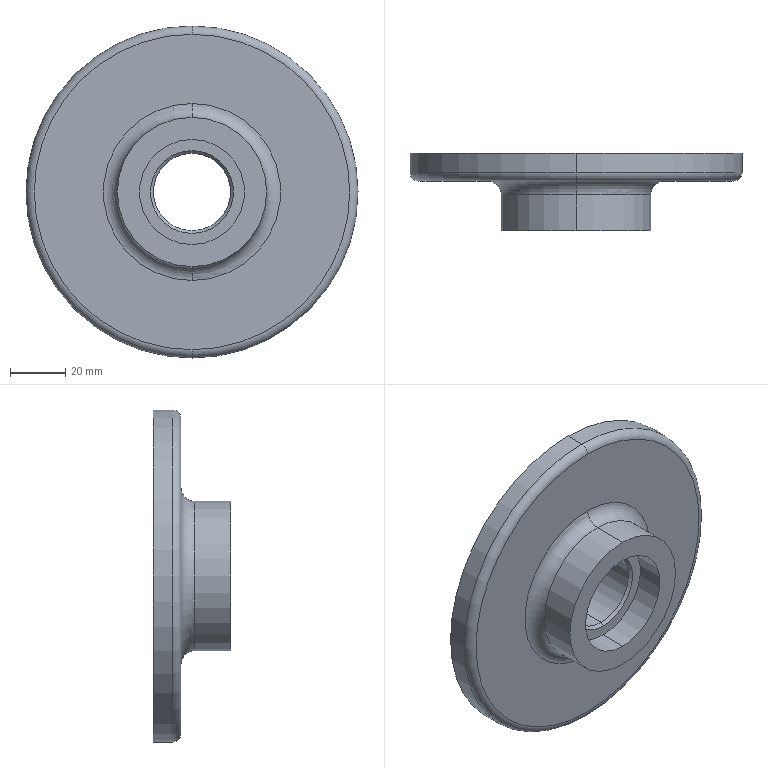Part | NX | features BREP 1 | 1 solid | 44 faces | box 120 x 27.99 x 120 mm | volume 131699 mm3 | cylinder 20 | cone 16 | torus 4 | plane 4 | commonest cylinder face diameters 3.3 x12 28 x2 38 x2 54 x2 120 x2
STEP:
#1=CARTESIAN_POINT('',(-56.,4.13,-1.65));
#2=VERTEX_POINT('',#1);
#3=CARTESIAN_POINT('',(-56.,4.13,1.65));
#4=VERTEX_POINT('',#3);
#5=CARTESIAN_POINT('',(-56.,4.13,0.));
#6=DIRECTION('',(0.,1.,0.));
#7=DIRECTION('',(0.,0.,1.));
#8=AXIS2_PLACEMENT_3D('',#5,#6,#7);
#9=CIRCLE('',#8,1.65);
#10=EDGE_CURVE('',#2,#4,#9,.T.);
#11=ORIENTED_EDGE('',*,*,#10,.F.);
#12=CARTESIAN_POINT('',(-56.,10.,-1.65));
#13=VERTEX_POINT('',#12);
#14=CARTESIAN_POINT('',(-56.,10.,-1.65));
#15=DIRECTION('',(0.,1.,0.));
#16=VECTOR('',#15,1000.);
#17=LINE('',#14,#16);
#18=EDGE_CURVE('',#2,#13,#17,.T.);
#19=ORIENTED_EDGE('',*,*,#18,.T.);
#20=CARTESIAN_POINT('',(-56.,10.,1.65));
#21=VERTEX_POINT('',#20);
#22=CARTESIAN_POINT('',(-56.,10.,0.));
#23=DIRECTION('',(0.,1.,0.));
#24=DIRECTION('',(0.,0.,1.));
#25=AXIS2_PLACEMENT_3D('',#22,#23,#24);
#26=CIRCLE('',#25,1.65);
#27=EDGE_CURVE('',#13,#21,#26,.T.);
#28=ORIENTED_EDGE('',*,*,#27,.T.);
#29=CARTESIAN_POINT('',(-56.,10.,1.65));
#30=DIRECTION('',(0.,1.,0.));
#31=VECTOR('',#30,1000.);
#32=LINE('',#29,#31);
#33=EDGE_CURVE('',#4,#21,#32,.T.);
#34=ORIENTED_EDGE('',*,*,#33,.F.);
#35=EDGE_LOOP('',(#11,#19,#28,#34));
#36=FACE_BOUND('',#35,.T.);
#37=CARTESIAN_POINT('',(-56.,10.,0.));
#38=DIRECTION('',(0.,1.,0.));
#39=DIRECTION('',(0.,0.,-1.));
#40=AXIS2_PLACEMENT_3D('',#37,#38,#39);
#41=CYLINDRICAL_SURFACE('',#40,1.65);
#42=ADVANCED_FACE('',(#36),#41,.F.);
#43=CARTESIAN_POINT('',(-56.,3.139,0.));
#44=VERTEX_POINT('',#43);
#45=CARTESIAN_POINT('',(-56.,4.13,1.65));
#46=DIRECTION('',(0.,0.515,0.8572));
#47=VECTOR('',#46,1000.);
#48=LINE('',#45,#47);
#49=EDGE_CURVE('',#44,#4,#48,.T.);
#50=ORIENTED_EDGE('',*,*,#49,.F.);
#51=CARTESIAN_POINT('',(-56.,4.13,-1.65));
#52=DIRECTION('',(0.,0.515,-0.8572));
#53=VECTOR('',#52,1000.);
#54=LINE('',#51,#53);
#55=EDGE_CURVE('',#44,#2,#54,.T.);
#56=ORIENTED_EDGE('',*,*,#55,.T.);
#57=ORIENTED_EDGE('',*,*,#10,.T.);
#58=EDGE_LOOP('',(#50,#56,#57));
#59=FACE_BOUND('',#58,.T.);
#60=CARTESIAN_POINT('',(-56.,4.13,0.));
#61=DIRECTION('',(0.,1.,0.));
#62=DIRECTION('',(0.,0.,-1.));
#63=AXIS2_PLACEMENT_3D('',#60,#61,#62);
#64=CONICAL_SURFACE('',#63,1.65,1.03);
#65=ADVANCED_FACE('',(#59),#64,.F.);
#66=CARTESIAN_POINT('',(-28.,4.13,-50.147));
#67=VERTEX_POINT('',#66);
#68=CARTESIAN_POINT('',(-28.,4.13,-46.847));
#69=VERTEX_POINT('',#68);
#70=CARTESIAN_POINT('',(-28.,4.13,-48.497));
#71=DIRECTION('',(0.,1.,0.));
#72=DIRECTION('',(0.,0.,1.));
#73=AXIS2_PLACEMENT_3D('',#70,#71,#72);
#74=CIRCLE('',#73,1.65);
#75=EDGE_CURVE('',#67,#69,#74,.T.);
#76=ORIENTED_EDGE('',*,*,#75,.F.);
#77=CARTESIAN_POINT('',(-28.,10.,-50.147));
#78=VERTEX_POINT('',#77);
#79=CARTESIAN_POINT('',(-28.,10.,-50.147));
#80=DIRECTION('',(0.,1.,0.));
#81=VECTOR('',#80,1000.);
#82=LINE('',#79,#81);
#83=EDGE_CURVE('',#67,#78,#82,.T.);
#84=ORIENTED_EDGE('',*,*,#83,.T.);
#85=CARTESIAN_POINT('',(-28.,10.,-46.847));
#86=VERTEX_POINT('',#85);
#87=CARTESIAN_POINT('',(-28.,10.,-48.497));
#88=DIRECTION('',(0.,1.,0.));
#89=DIRECTION('',(0.,0.,1.));
#90=AXIS2_PLACEMENT_3D('',#87,#88,#89);
#91=CIRCLE('',#90,1.65);
#92=EDGE_CURVE('',#78,#86,#91,.T.);
#93=ORIENTED_EDGE('',*,*,#92,.T.);
#94=CARTESIAN_POINT('',(-28.,10.,-46.847));
#95=DIRECTION('',(0.,1.,0.));
#96=VECTOR('',#95,1000.);
#97=LINE('',#94,#96);
#98=EDGE_CURVE('',#69,#86,#97,.T.);
#99=ORIENTED_EDGE('',*,*,#98,.F.);
#100=EDGE_LOOP('',(#76,#84,#93,#99));
#101=FACE_BOUND('',#100,.T.);
#102=CARTESIAN_POINT('',(-28.,10.,-48.497));
#103=DIRECTION('',(0.,1.,0.));
#104=DIRECTION('',(0.,0.,-1.));
#105=AXIS2_PLACEMENT_3D('',#102,#103,#104);
#106=CYLINDRICAL_SURFACE('',#105,1.65);
#107=ADVANCED_FACE('',(#101),#106,.F.);
#108=CARTESIAN_POINT('',(-28.,3.139,-48.497));
#109=VERTEX_POINT('',#108);
#110=CARTESIAN_POINT('',(-28.,4.13,-46.847));
#111=DIRECTION('',(0.,0.515,0.8572));
#112=VECTOR('',#111,1000.);
#113=LINE('',#110,#112);
#114=EDGE_CURVE('',#109,#69,#113,.T.);
#115=ORIENTED_EDGE('',*,*,#114,.F.);
#116=CARTESIAN_POINT('',(-28.,4.13,-50.147));
#117=DIRECTION('',(0.,0.515,-0.8572));
#118=VECTOR('',#117,1000.);
#119=LINE('',#116,#118);
#120=EDGE_CURVE('',#109,#67,#119,.T.);
#121=ORIENTED_EDGE('',*,*,#120,.T.);
#122=ORIENTED_EDGE('',*,*,#75,.T.);
#123=EDGE_LOOP('',(#115,#121,#122));
#124=FACE_BOUND('',#123,.T.);
#125=CARTESIAN_POINT('',(-28.,4.13,-48.497));
#126=DIRECTION('',(0.,1.,0.));
#127=DIRECTION('',(0.,0.,-1.));
#128=AXIS2_PLACEMENT_3D('',#125,#126,#127);
#129=CONICAL_SURFACE('',#128,1.65,1.03);
#130=ADVANCED_FACE('',(#124),#129,.F.);
#131=CARTESIAN_POINT('',(28.,4.13,-50.147));
#132=VERTEX_POINT('',#131);
#133=CARTESIAN_POINT('',(28.,4.13,-46.847));
#134=VERTEX_POINT('',#133);
#135=CARTESIAN_POINT('',(28.,4.13,-48.497));
#136=DIRECTION('',(0.,1.,0.));
#137=DIRECTION('',(0.,0.,1.));
#138=AXIS2_PLACEMENT_3D('',#135,#136,#137);
#139=CIRCLE('',#138,1.65);
#140=EDGE_CURVE('',#132,#134,#139,.T.);
#141=ORIENTED_EDGE('',*,*,#140,.F.);
#142=CARTESIAN_POINT('',(28.,10.,-50.147));
#143=VERTEX_POINT('',#142);
#144=CARTESIAN_POINT('',(28.,10.,-50.147));
#145=DIRECTION('',(0.,1.,0.));
#146=VECTOR('',#145,1000.);
#147=LINE('',#144,#146);
#148=EDGE_CURVE('',#132,#143,#147,.T.);
#149=ORIENTED_EDGE('',*,*,#148,.T.);
#150=CARTESIAN_POINT('',(28.,10.,-46.847));
#151=VERTEX_POINT('',#150);
#152=CARTESIAN_POINT('',(28.,10.,-48.497));
#153=DIRECTION('',(0.,1.,0.));
#154=DIRECTION('',(0.,0.,1.));
#155=AXIS2_PLACEMENT_3D('',#152,#153,#154);
#156=CIRCLE('',#155,1.65);
#157=EDGE_CURVE('',#143,#151,#156,.T.);
#158=ORIENTED_EDGE('',*,*,#157,.T.);
#159=CARTESIAN_POINT('',(28.,10.,-46.847));
#160=DIRECTION('',(0.,1.,0.));
#161=VECTOR('',#160,1000.);
#162=LINE('',#159,#161);
#163=EDGE_CURVE('',#134,#151,#162,.T.);
#164=ORIENTED_EDGE('',*,*,#163,.F.);
#165=EDGE_LOOP('',(#141,#149,#158,#164));
#166=FACE_BOUND('',#165,.T.);
#167=CARTESIAN_POINT('',(28.,10.,-48.497));
#168=DIRECTION('',(0.,1.,0.));
#169=DIRECTION('',(0.,0.,-1.));
#170=AXIS2_PLACEMENT_3D('',#167,#168,#169);
#171=CYLINDRICAL_SURFACE('',#170,1.65);
#172=ADVANCED_FACE('',(#166),#171,.F.);
#173=CARTESIAN_POINT('',(28.,3.139,-48.497));
#174=VERTEX_POINT('',#173);
#175=CARTESIAN_POINT('',(28.,4.13,-46.847));
#176=DIRECTION('',(0.,0.515,0.8572));
#177=VECTOR('',#176,1000.);
#178=LINE('',#175,#177);
#179=EDGE_CURVE('',#174,#134,#178,.T.);
#180=ORIENTED_EDGE('',*,*,#179,.F.);
#181=CARTESIAN_POINT('',(28.,4.13,-50.147));
#182=DIRECTION('',(0.,0.515,-0.8572));
#183=VECTOR('',#182,1000.);
#184=LINE('',#181,#183);
#185=EDGE_CURVE('',#174,#132,#184,.T.);
#186=ORIENTED_EDGE('',*,*,#185,.T.);
#187=ORIENTED_EDGE('',*,*,#140,.T.);
#188=EDGE_LOOP('',(#180,#186,#187));
#189=FACE_BOUND('',#188,.T.);
#190=CARTESIAN_POINT('',(28.,4.13,-48.497));
#191=DIRECTION('',(0.,1.,0.));
#192=DIRECTION('',(0.,0.,-1.));
#193=AXIS2_PLACEMENT_3D('',#190,#191,#192);
#194=CONICAL_SURFACE('',#193,1.65,1.03);
#195=ADVANCED_FACE('',(#189),#194,.F.);
#196=CARTESIAN_POINT('',(56.,4.13,-1.65));
#197=VERTEX_POINT('',#196);
#198=CARTESIAN_POINT('',(56.,4.13,1.65));
#199=VERTEX_POINT('',#198);
#200=CARTESIAN_POINT('',(56.,4.13,0.));
#201=DIRECTION('',(0.,1.,0.));
#202=DIRECTION('',(0.,0.,1.));
#203=AXIS2_PLACEMENT_3D('',#200,#201,#202);
#204=CIRCLE('',#203,1.65);
#205=EDGE_CURVE('',#197,#199,#204,.T.);
#206=ORIENTED_EDGE('',*,*,#205,.F.);
#207=CARTESIAN_POINT('',(56.,10.,-1.65));
#208=VERTEX_POINT('',#207);
#209=CARTESIAN_POINT('',(56.,10.,-1.65));
#210=DIRECTION('',(0.,1.,0.));
#211=VECTOR('',#210,1000.);
#212=LINE('',#209,#211);
#213=EDGE_CURVE('',#197,#208,#212,.T.);
#214=ORIENTED_EDGE('',*,*,#213,.T.);
#215=CARTESIAN_POINT('',(56.,10.,1.65));
#216=VERTEX_POINT('',#215);
#217=CARTESIAN_POINT('',(56.,10.,0.));
#218=DIRECTION('',(0.,1.,0.));
#219=DIRECTION('',(0.,0.,1.));
#220=AXIS2_PLACEMENT_3D('',#217,#218,#219);
#221=CIRCLE('',#220,1.65);
#222=EDGE_CURVE('',#208,#216,#221,.T.);
#223=ORIENTED_EDGE('',*,*,#222,.T.);
#224=CARTESIAN_POINT('',(56.,10.,1.65));
#225=DIRECTION('',(0.,1.,0.));
#226=VECTOR('',#225,1000.);
#227=LINE('',#224,#226);
#228=EDGE_CURVE('',#199,#216,#227,.T.);
#229=ORIENTED_EDGE('',*,*,#228,.F.);
#230=EDGE_LOOP('',(#206,#214,#223,#229));
#231=FACE_BOUND('',#230,.T.);
#232=CARTESIAN_POINT('',(56.,10.,0.));
#233=DIRECTION('',(0.,1.,0.));
#234=DIRECTION('',(0.,0.,-1.));
#235=AXIS2_PLACEMENT_3D('',#232,#233,#234);
#236=CYLINDRICAL_SURFACE('',#235,1.65);
#237=ADVANCED_FACE('',(#231),#236,.F.);
#238=CARTESIAN_POINT('',(56.,3.139,0.));
#239=VERTEX_POINT('',#238);
#240=CARTESIAN_POINT('',(56.,4.13,1.65));
#241=DIRECTION('',(0.,0.515,0.8572));
#242=VECTOR('',#241,1000.);
#243=LINE('',#240,#242);
#244=EDGE_CURVE('',#239,#199,#243,.T.);
#245=ORIENTED_EDGE('',*,*,#244,.F.);
#246=CARTESIAN_POINT('',(56.,4.13,-1.65));
#247=DIRECTION('',(0.,0.515,-0.8572));
#248=VECTOR('',#247,1000.);
#249=LINE('',#246,#248);
#250=EDGE_CURVE('',#239,#197,#249,.T.);
#251=ORIENTED_EDGE('',*,*,#250,.T.);
#252=ORIENTED_EDGE('',*,*,#205,.T.);
#253=EDGE_LOOP('',(#245,#251,#252));
#254=FACE_BOUND('',#253,.T.);
#255=CARTESIAN_POINT('',(56.,4.13,0.));
#256=DIRECTION('',(0.,1.,0.));
#257=DIRECTION('',(0.,0.,-1.));
#258=AXIS2_PLACEMENT_3D('',#255,#256,#257);
#259=CONICAL_SURFACE('',#258,1.65,1.03);
#260=ADVANCED_FACE('',(#254),#259,.F.);
#261=CARTESIAN_POINT('',(28.,4.13,46.847));
#262=VERTEX_POINT('',#261);
#263=CARTESIAN_POINT('',(28.,4.13,50.147));
#264=VERTEX_POINT('',#263);
#265=CARTESIAN_POINT('',(28.,4.13,48.497));
#266=DIRECTION('',(0.,1.,0.));
#267=DIRECTION('',(0.,0.,1.));
#268=AXIS2_PLACEMENT_3D('',#265,#266,#267);
#269=CIRCLE('',#268,1.65);
#270=EDGE_CURVE('',#262,#264,#269,.T.);
#271=ORIENTED_EDGE('',*,*,#270,.F.);
#272=CARTESIAN_POINT('',(28.,10.,46.847));
#273=VERTEX_POINT('',#272);
#274=CARTESIAN_POINT('',(28.,10.,46.847));
#275=DIRECTION('',(0.,1.,0.));
#276=VECTOR('',#275,1000.);
#277=LINE('',#274,#276);
#278=EDGE_CURVE('',#262,#273,#277,.T.);
#279=ORIENTED_EDGE('',*,*,#278,.T.);
#280=CARTESIAN_POINT('',(28.,10.,50.147));
#281=VERTEX_POINT('',#280);
#282=CARTESIAN_POINT('',(28.,10.,48.497));
#283=DIRECTION('',(0.,1.,0.));
#284=DIRECTION('',(0.,0.,1.));
#285=AXIS2_PLACEMENT_3D('',#282,#283,#284);
#286=CIRCLE('',#285,1.65);
#287=EDGE_CURVE('',#273,#281,#286,.T.);
#288=ORIENTED_EDGE('',*,*,#287,.T.);
#289=CARTESIAN_POINT('',(28.,10.,50.147));
#290=DIRECTION('',(0.,1.,0.));
#291=VECTOR('',#290,1000.);
#292=LINE('',#289,#291);
#293=EDGE_CURVE('',#264,#281,#292,.T.);
#294=ORIENTED_EDGE('',*,*,#293,.F.);
#295=EDGE_LOOP('',(#271,#279,#288,#294));
#296=FACE_BOUND('',#295,.T.);
#297=CARTESIAN_POINT('',(28.,10.,48.497));
#298=DIRECTION('',(0.,1.,0.));
#299=DIRECTION('',(0.,0.,-1.));
#300=AXIS2_PLACEMENT_3D('',#297,#298,#299);
#301=CYLINDRICAL_SURFACE('',#300,1.65);
#302=ADVANCED_FACE('',(#296),#301,.F.);
#303=CARTESIAN_POINT('',(28.,3.139,48.497));
#304=VERTEX_POINT('',#303);
#305=CARTESIAN_POINT('',(28.,4.13,50.147));
#306=DIRECTION('',(0.,0.515,0.8572));
#307=VECTOR('',#306,1000.);
#308=LINE('',#305,#307);
#309=EDGE_CURVE('',#304,#264,#308,.T.);
#310=ORIENTED_EDGE('',*,*,#309,.F.);
#311=CARTESIAN_POINT('',(28.,4.13,46.847));
#312=DIRECTION('',(0.,0.515,-0.8572));
#313=VECTOR('',#312,1000.);
#314=LINE('',#311,#313);
#315=EDGE_CURVE('',#304,#262,#314,.T.);
#316=ORIENTED_EDGE('',*,*,#315,.T.);
#317=ORIENTED_EDGE('',*,*,#270,.T.);
#318=EDGE_LOOP('',(#310,#316,#317));
#319=FACE_BOUND('',#318,.T.);
#320=CARTESIAN_POINT('',(28.,4.13,48.497));
#321=DIRECTION('',(0.,1.,0.));
#322=DIRECTION('',(0.,0.,-1.));
#323=AXIS2_PLACEMENT_3D('',#320,#321,#322);
#324=CONICAL_SURFACE('',#323,1.65,1.03);
#325=ADVANCED_FACE('',(#319),#324,.F.);
#326=CARTESIAN_POINT('',(-28.,4.13,46.847));
#327=VERTEX_POINT('',#326);
#328=CARTESIAN_POINT('',(-28.,4.13,50.147));
#329=VERTEX_POINT('',#328);
#330=CARTESIAN_POINT('',(-28.,4.13,48.497));
#331=DIRECTION('',(0.,1.,0.));
#332=DIRECTION('',(0.,0.,1.));
#333=AXIS2_PLACEMENT_3D('',#330,#331,#332);
#334=CIRCLE('',#333,1.65);
#335=EDGE_CURVE('',#327,#329,#334,.T.);
#336=ORIENTED_EDGE('',*,*,#335,.F.);
#337=CARTESIAN_POINT('',(-28.,10.,46.847));
#338=VERTEX_POINT('',#337);
#339=CARTESIAN_POINT('',(-28.,10.,46.847));
#340=DIRECTION('',(0.,1.,0.));
#341=VECTOR('',#340,1000.);
#342=LINE('',#339,#341);
#343=EDGE_CURVE('',#327,#338,#342,.T.);
#344=ORIENTED_EDGE('',*,*,#343,.T.);
#345=CARTESIAN_POINT('',(-28.,10.,50.147));
#346=VERTEX_POINT('',#345);
#347=CARTESIAN_POINT('',(-28.,10.,48.497));
#348=DIRECTION('',(0.,1.,0.));
#349=DIRECTION('',(0.,0.,1.));
#350=AXIS2_PLACEMENT_3D('',#347,#348,#349);
#351=CIRCLE('',#350,1.65);
#352=EDGE_CURVE('',#338,#346,#351,.T.);
#353=ORIENTED_EDGE('',*,*,#352,.T.);
#354=CARTESIAN_POINT('',(-28.,10.,50.147));
#355=DIRECTION('',(0.,1.,0.));
#356=VECTOR('',#355,1000.);
#357=LINE('',#354,#356);
#358=EDGE_CURVE('',#329,#346,#357,.T.);
#359=ORIENTED_EDGE('',*,*,#358,.F.);
#360=EDGE_LOOP('',(#336,#344,#353,#359));
#361=FACE_BOUND('',#360,.T.);
#362=CARTESIAN_POINT('',(-28.,10.,48.497));
#363=DIRECTION('',(0.,1.,0.));
#364=DIRECTION('',(0.,0.,-1.));
#365=AXIS2_PLACEMENT_3D('',#362,#363,#364);
#366=CYLINDRICAL_SURFACE('',#365,1.65);
#367=ADVANCED_FACE('',(#361),#366,.F.);
#368=CARTESIAN_POINT('',(-28.,3.139,48.497));
#369=VERTEX_POINT('',#368);
#370=CARTESIAN_POINT('',(-28.,4.13,50.147));
#371=DIRECTION('',(0.,0.515,0.8572));
#372=VECTOR('',#371,1000.);
#373=LINE('',#370,#372);
#374=EDGE_CURVE('',#369,#329,#373,.T.);
#375=ORIENTED_EDGE('',*,*,#374,.F.);
#376=CARTESIAN_POINT('',(-28.,4.13,46.847));
#377=DIRECTION('',(0.,0.515,-0.8572));
#378=VECTOR('',#377,1000.);
#379=LINE('',#376,#378);
#380=EDGE_CURVE('',#369,#327,#379,.T.);
#381=ORIENTED_EDGE('',*,*,#380,.T.);
#382=ORIENTED_EDGE('',*,*,#335,.T.);
#383=EDGE_LOOP('',(#375,#381,#382));
#384=FACE_BOUND('',#383,.T.);
#385=CARTESIAN_POINT('',(-28.,4.13,48.497));
#386=DIRECTION('',(0.,1.,0.));
#387=DIRECTION('',(0.,0.,-1.));
#388=AXIS2_PLACEMENT_3D('',#385,#386,#387);
#389=CONICAL_SURFACE('',#388,1.65,1.03);
#390=ADVANCED_FACE('',(#384),#389,.F.);
#391=CARTESIAN_POINT('',(0.,0.,57.));
#392=VERTEX_POINT('',#391);
#393=CARTESIAN_POINT('',(0.,0.,-57.));
#394=VERTEX_POINT('',#393);
#395=CARTESIAN_POINT('',(0.,0.,0.));
#396=DIRECTION('',(0.,1.,0.));
#397=DIRECTION('',(0.,0.,1.));
#398=AXIS2_PLACEMENT_3D('',#395,#396,#397);
#399=CIRCLE('',#398,57.);
#400=EDGE_CURVE('',#392,#394,#399,.T.);
#401=ORIENTED_EDGE('',*,*,#400,.T.);
#402=CARTESIAN_POINT('',(0.,3.,-60.));
#403=VERTEX_POINT('',#402);
#404=CARTESIAN_POINT('',(0.,3.,-57.));
#405=DIRECTION('',(1.,0.,0.));
#406=DIRECTION('',(0.,0.,-1.));
#407=AXIS2_PLACEMENT_3D('',#404,#405,#406);
#408=CIRCLE('',#407,3.);
#409=EDGE_CURVE('',#394,#403,#408,.T.);
#410=ORIENTED_EDGE('',*,*,#409,.T.);
#411=CARTESIAN_POINT('',(0.,3.,60.));
#412=VERTEX_POINT('',#411);
#413=CARTESIAN_POINT('',(0.,3.,0.));
#414=DIRECTION('',(0.,1.,0.));
#415=DIRECTION('',(0.,0.,1.));
#416=AXIS2_PLACEMENT_3D('',#413,#414,#415);
#417=CIRCLE('',#416,60.);
#418=EDGE_CURVE('',#412,#403,#417,.T.);
#419=ORIENTED_EDGE('',*,*,#418,.F.);
#420=CARTESIAN_POINT('',(0.,3.,57.));
#421=DIRECTION('',(-1.,0.,0.));
#422=DIRECTION('',(0.,0.,1.));
#423=AXIS2_PLACEMENT_3D('',#420,#421,#422);
#424=CIRCLE('',#423,3.);
#425=EDGE_CURVE('',#392,#412,#424,.T.);
#426=ORIENTED_EDGE('',*,*,#425,.F.);
#427=EDGE_LOOP('',(#401,#410,#419,#426));
#428=FACE_BOUND('',#427,.T.);
#429=CARTESIAN_POINT('',(0.,3.,0.));
#430=DIRECTION('',(0.,1.,0.));
#431=DIRECTION('',(0.,0.,-1.));
#432=AXIS2_PLACEMENT_3D('',#429,#430,#431);
#433=TOROIDAL_SURFACE('',#432,57.,3.);
#434=ADVANCED_FACE('',(#428),#433,.T.);
#435=CARTESIAN_POINT('',(0.,0.,-32.));
#436=VERTEX_POINT('',#435);
#437=CARTESIAN_POINT('',(0.,0.,32.));
#438=VERTEX_POINT('',#437);
#439=CARTESIAN_POINT('',(0.,0.,0.));
#440=DIRECTION('',(0.,1.,0.));
#441=DIRECTION('',(0.,0.,1.));
#442=AXIS2_PLACEMENT_3D('',#439,#440,#441);
#443=CIRCLE('',#442,32.);
#444=EDGE_CURVE('',#436,#438,#443,.T.);
#445=ORIENTED_EDGE('',*,*,#444,.F.);
#446=CARTESIAN_POINT('',(0.,-5.,-27.));
#447=VERTEX_POINT('',#446);
#448=CARTESIAN_POINT('',(0.,-5.,-32.));
#449=DIRECTION('',(1.,0.,0.));
#450=DIRECTION('',(0.,0.,-1.));
#451=AXIS2_PLACEMENT_3D('',#448,#449,#450);
#452=CIRCLE('',#451,5.);
#453=EDGE_CURVE('',#436,#447,#452,.T.);
#454=ORIENTED_EDGE('',*,*,#453,.T.);
#455=CARTESIAN_POINT('',(0.,-5.,27.));
#456=VERTEX_POINT('',#455);
#457=CARTESIAN_POINT('',(0.,-5.,0.));
#458=DIRECTION('',(0.,1.,0.));
#459=DIRECTION('',(0.,0.,1.));
#460=AXIS2_PLACEMENT_3D('',#457,#458,#459);
#461=CIRCLE('',#460,27.);
#462=EDGE_CURVE('',#447,#456,#461,.T.);
#463=ORIENTED_EDGE('',*,*,#462,.T.);
#464=CARTESIAN_POINT('',(0.,-5.,32.));
#465=DIRECTION('',(-1.,0.,0.));
#466=DIRECTION('',(0.,0.,1.));
#467=AXIS2_PLACEMENT_3D('',#464,#465,#466);
#468=CIRCLE('',#467,5.);
#469=EDGE_CURVE('',#438,#456,#468,.T.);
#470=ORIENTED_EDGE('',*,*,#469,.F.);
#471=EDGE_LOOP('',(#445,#454,#463,#470));
#472=FACE_BOUND('',#471,.T.);
#473=CARTESIAN_POINT('',(0.,-5.,0.));
#474=DIRECTION('',(0.,1.,0.));
#475=DIRECTION('',(0.,0.,-1.));
#476=AXIS2_PLACEMENT_3D('',#473,#474,#475);
#477=TOROIDAL_SURFACE('',#476,32.,5.);
#478=ADVANCED_FACE('',(#472),#477,.F.);
#479=CARTESIAN_POINT('',(0.,-17.99,27.));
#480=VERTEX_POINT('',#479);
#481=CARTESIAN_POINT('',(0.,-17.99,-27.));
#482=VERTEX_POINT('',#481);
#483=CARTESIAN_POINT('',(0.,-17.99,0.));
#484=DIRECTION('',(0.,1.,0.));
#485=DIRECTION('',(0.,0.,1.));
#486=AXIS2_PLACEMENT_3D('',#483,#484,#485);
#487=CIRCLE('',#486,27.);
#488=EDGE_CURVE('',#480,#482,#487,.T.);
#489=ORIENTED_EDGE('',*,*,#488,.T.);
#490=CARTESIAN_POINT('',(0.,39.293,-27.));
#491=DIRECTION('',(0.,1.,0.));
#492=VECTOR('',#491,1000.);
#493=LINE('',#490,#492);
#494=EDGE_CURVE('',#482,#447,#493,.T.);
#495=ORIENTED_EDGE('',*,*,#494,.T.);
#496=CARTESIAN_POINT('',(0.,-5.,0.));
#497=DIRECTION('',(0.,1.,0.));
#498=DIRECTION('',(0.,0.,1.));
#499=AXIS2_PLACEMENT_3D('',#496,#497,#498);
#500=CIRCLE('',#499,27.);
#501=EDGE_CURVE('',#456,#447,#500,.T.);
#502=ORIENTED_EDGE('',*,*,#501,.F.);
#503=CARTESIAN_POINT('',(0.,39.293,27.));
#504=DIRECTION('',(0.,1.,0.));
#505=VECTOR('',#504,1000.);
#506=LINE('',#503,#505);
#507=EDGE_CURVE('',#480,#456,#506,.T.);
#508=ORIENTED_EDGE('',*,*,#507,.F.);
#509=EDGE_LOOP('',(#489,#495,#502,#508));
#510=FACE_BOUND('',#509,.T.);
#511=CARTESIAN_POINT('',(0.,39.293,0.));
#512=DIRECTION('',(0.,1.,0.));
#513=DIRECTION('',(0.,0.,-1.));
#514=AXIS2_PLACEMENT_3D('',#511,#512,#513);
#515=CYLINDRICAL_SURFACE('',#514,27.);
#516=ADVANCED_FACE('',(#510),#515,.T.);
#517=CARTESIAN_POINT('',(0.,-17.99,-19.));
#518=VERTEX_POINT('',#517);
#519=CARTESIAN_POINT('',(0.,-17.99,19.));
#520=VERTEX_POINT('',#519);
#521=CARTESIAN_POINT('',(0.,-17.99,0.));
#522=DIRECTION('',(0.,1.,0.));
#523=DIRECTION('',(0.,0.,1.));
#524=AXIS2_PLACEMENT_3D('',#521,#522,#523);
#525=CIRCLE('',#524,19.);
#526=EDGE_CURVE('',#518,#520,#525,.T.);
#527=ORIENTED_EDGE('',*,*,#526,.F.);
#528=CARTESIAN_POINT('',(0.,-7.99,-19.));
#529=VERTEX_POINT('',#528);
#530=CARTESIAN_POINT('',(0.,39.293,-19.));
#531=DIRECTION('',(0.,1.,0.));
#532=VECTOR('',#531,1000.);
#533=LINE('',#530,#532);
#534=EDGE_CURVE('',#518,#529,#533,.T.);
#535=ORIENTED_EDGE('',*,*,#534,.T.);
#536=CARTESIAN_POINT('',(0.,-7.99,19.));
#537=VERTEX_POINT('',#536);
#538=CARTESIAN_POINT('',(0.,-7.99,0.));
#539=DIRECTION('',(0.,1.,0.));
#540=DIRECTION('',(0.,0.,1.));
#541=AXIS2_PLACEMENT_3D('',#538,#539,#540);
#542=CIRCLE('',#541,19.);
#543=EDGE_CURVE('',#529,#537,#542,.T.);
#544=ORIENTED_EDGE('',*,*,#543,.T.);
#545=CARTESIAN_POINT('',(0.,39.293,19.));
#546=DIRECTION('',(0.,1.,0.));
#547=VECTOR('',#546,1000.);
#548=LINE('',#545,#547);
#549=EDGE_CURVE('',#520,#537,#548,.T.);
#550=ORIENTED_EDGE('',*,*,#549,.F.);
#551=EDGE_LOOP('',(#527,#535,#544,#550));
#552=FACE_BOUND('',#551,.T.);
#553=CARTESIAN_POINT('',(0.,39.293,0.));
#554=DIRECTION('',(0.,1.,0.));
#555=DIRECTION('',(0.,0.,-1.));
#556=AXIS2_PLACEMENT_3D('',#553,#554,#555);
#557=CYLINDRICAL_SURFACE('',#556,19.);
#558=ADVANCED_FACE('',(#552),#557,.F.);
#559=CARTESIAN_POINT('',(0.,-6.99,-14.));
#560=VERTEX_POINT('',#559);
#561=CARTESIAN_POINT('',(0.,-6.99,14.));
#562=VERTEX_POINT('',#561);
#563=CARTESIAN_POINT('',(0.,-6.99,0.));
#564=DIRECTION('',(0.,1.,0.));
#565=DIRECTION('',(0.,0.,1.));
#566=AXIS2_PLACEMENT_3D('',#563,#564,#565);
#567=CIRCLE('',#566,14.);
#568=EDGE_CURVE('',#560,#562,#567,.T.);
#569=ORIENTED_EDGE('',*,*,#568,.T.);
#570=CARTESIAN_POINT('',(0.,-7.99,15.));
#571=VERTEX_POINT('',#570);
#572=CARTESIAN_POINT('',(0.,-6.99,14.));
#573=DIRECTION('',(0.,-0.7071,0.7071));
#574=VECTOR('',#573,1000.);
#575=LINE('',#572,#574);
#576=EDGE_CURVE('',#571,#562,#575,.F.);
#577=ORIENTED_EDGE('',*,*,#576,.F.);
#578=CARTESIAN_POINT('',(0.,-7.99,-15.));
#579=VERTEX_POINT('',#578);
#580=CARTESIAN_POINT('',(0.,-7.99,0.));
#581=DIRECTION('',(0.,1.,0.));
#582=DIRECTION('',(0.,0.,1.));
#583=AXIS2_PLACEMENT_3D('',#580,#581,#582);
#584=CIRCLE('',#583,15.);
#585=EDGE_CURVE('',#579,#571,#584,.T.);
#586=ORIENTED_EDGE('',*,*,#585,.F.);
#587=CARTESIAN_POINT('',(0.,-6.99,-14.));
#588=DIRECTION('',(0.,-0.7071,-0.7071));
#589=VECTOR('',#588,1000.);
#590=LINE('',#587,#589);
#591=EDGE_CURVE('',#579,#560,#590,.F.);
#592=ORIENTED_EDGE('',*,*,#591,.T.);
#593=EDGE_LOOP('',(#569,#577,#586,#592));
#594=FACE_BOUND('',#593,.T.);
#595=CARTESIAN_POINT('',(0.,-6.99,0.));
#596=DIRECTION('',(0.,-1.,0.));
#597=DIRECTION('',(0.,0.,1.));
#598=AXIS2_PLACEMENT_3D('',#595,#596,#597);
#599=CONICAL_SURFACE('',#598,14.,0.7854);
#600=ADVANCED_FACE('',(#594),#599,.F.);
#601=ORIENTED_EDGE('',*,*,#568,.F.);
#602=CARTESIAN_POINT('',(0.,9.,-14.));
#603=VERTEX_POINT('',#602);
#604=CARTESIAN_POINT('',(0.,39.293,-14.));
#605=DIRECTION('',(0.,1.,0.));
#606=VECTOR('',#605,1000.);
#607=LINE('',#604,#606);
#608=EDGE_CURVE('',#560,#603,#607,.T.);
#609=ORIENTED_EDGE('',*,*,#608,.T.);
#610=CARTESIAN_POINT('',(0.,9.,14.));
#611=VERTEX_POINT('',#610);
#612=CARTESIAN_POINT('',(0.,9.,0.));
#613=DIRECTION('',(0.,1.,0.));
#614=DIRECTION('',(0.,0.,1.));
#615=AXIS2_PLACEMENT_3D('',#612,#613,#614);
#616=CIRCLE('',#615,14.);
#617=EDGE_CURVE('',#603,#611,#616,.T.);
#618=ORIENTED_EDGE('',*,*,#617,.T.);
#619=CARTESIAN_POINT('',(0.,39.293,14.));
#620=DIRECTION('',(0.,1.,0.));
#621=VECTOR('',#620,1000.);
#622=LINE('',#619,#621);
#623=EDGE_CURVE('',#562,#611,#622,.T.);
#624=ORIENTED_EDGE('',*,*,#623,.F.);
#625=EDGE_LOOP('',(#601,#609,#618,#624));
#626=FACE_BOUND('',#625,.T.);
#627=CARTESIAN_POINT('',(0.,39.293,0.));
#628=DIRECTION('',(0.,1.,0.));
#629=DIRECTION('',(0.,0.,-1.));
#630=AXIS2_PLACEMENT_3D('',#627,#628,#629);
#631=CYLINDRICAL_SURFACE('',#630,14.);
#632=ADVANCED_FACE('',(#626),#631,.F.);
#633=ORIENTED_EDGE('',*,*,#617,.F.);
#634=CARTESIAN_POINT('',(0.,10.,-15.));
#635=VERTEX_POINT('',#634);
#636=CARTESIAN_POINT('',(0.,10.,-15.));
#637=DIRECTION('',(0.,0.7071,-0.7071));
#638=VECTOR('',#637,1000.);
#639=LINE('',#636,#638);
#640=EDGE_CURVE('',#603,#635,#639,.T.);
#641=ORIENTED_EDGE('',*,*,#640,.T.);
#642=CARTESIAN_POINT('',(0.,10.,15.));
#643=VERTEX_POINT('',#642);
#644=CARTESIAN_POINT('',(0.,10.,0.));
#645=DIRECTION('',(0.,1.,0.));
#646=DIRECTION('',(0.,0.,1.));
#647=AXIS2_PLACEMENT_3D('',#644,#645,#646);
#648=CIRCLE('',#647,15.);
#649=EDGE_CURVE('',#635,#643,#648,.T.);
#650=ORIENTED_EDGE('',*,*,#649,.T.);
#651=CARTESIAN_POINT('',(0.,10.,15.));
#652=DIRECTION('',(0.,0.7071,0.7071));
#653=VECTOR('',#652,1000.);
#654=LINE('',#651,#653);
#655=EDGE_CURVE('',#611,#643,#654,.T.);
#656=ORIENTED_EDGE('',*,*,#655,.F.);
#657=EDGE_LOOP('',(#633,#641,#650,#656));
#658=FACE_BOUND('',#657,.T.);
#659=CARTESIAN_POINT('',(0.,10.,0.));
#660=DIRECTION('',(0.,1.,0.));
#661=DIRECTION('',(0.,0.,-1.));
#662=AXIS2_PLACEMENT_3D('',#659,#660,#661);
#663=CONICAL_SURFACE('',#662,15.,0.7854);
#664=ADVANCED_FACE('',(#658),#663,.F.);
#665=ORIENTED_EDGE('',*,*,#418,.T.);
#666=CARTESIAN_POINT('',(0.,10.,-60.));
#667=VERTEX_POINT('',#666);
#668=CARTESIAN_POINT('',(0.,39.293,-60.));
#669=DIRECTION('',(0.,1.,0.));
#670=VECTOR('',#669,1000.);
#671=LINE('',#668,#670);
#672=EDGE_CURVE('',#403,#667,#671,.T.);
#673=ORIENTED_EDGE('',*,*,#672,.T.);
#674=CARTESIAN_POINT('',(0.,10.,60.));
#675=VERTEX_POINT('',#674);
#676=CARTESIAN_POINT('',(0.,10.,0.));
#677=DIRECTION('',(0.,1.,0.));
#678=DIRECTION('',(0.,0.,1.));
#679=AXIS2_PLACEMENT_3D('',#676,#677,#678);
#680=CIRCLE('',#679,60.);
#681=EDGE_CURVE('',#675,#667,#680,.T.);
#682=ORIENTED_EDGE('',*,*,#681,.F.);
#683=CARTESIAN_POINT('',(0.,39.293,60.));
#684=DIRECTION('',(0.,1.,0.));
#685=VECTOR('',#684,1000.);
#686=LINE('',#683,#685);
#687=EDGE_CURVE('',#412,#675,#686,.T.);
#688=ORIENTED_EDGE('',*,*,#687,.F.);
#689=EDGE_LOOP('',(#665,#673,#682,#688));
#690=FACE_BOUND('',#689,.T.);
#691=CARTESIAN_POINT('',(0.,39.293,0.));
#692=DIRECTION('',(0.,1.,0.));
#693=DIRECTION('',(0.,0.,-1.));
#694=AXIS2_PLACEMENT_3D('',#691,#692,#693);
#695=CYLINDRICAL_SURFACE('',#694,60.);
#696=ADVANCED_FACE('',(#690),#695,.T.);
#697=ORIENTED_EDGE('',*,*,#672,.F.);
#698=CARTESIAN_POINT('',(0.,3.,0.));
#699=DIRECTION('',(0.,1.,0.));
#700=DIRECTION('',(0.,0.,1.));
#701=AXIS2_PLACEMENT_3D('',#698,#699,#700);
#702=CIRCLE('',#701,60.);
#703=EDGE_CURVE('',#403,#412,#702,.T.);
#704=ORIENTED_EDGE('',*,*,#703,.T.);
#705=ORIENTED_EDGE('',*,*,#687,.T.);
#706=CARTESIAN_POINT('',(0.,10.,0.));
#707=DIRECTION('',(0.,1.,0.));
#708=DIRECTION('',(0.,0.,1.));
#709=AXIS2_PLACEMENT_3D('',#706,#707,#708);
#710=CIRCLE('',#709,60.);
#711=EDGE_CURVE('',#667,#675,#710,.T.);
#712=ORIENTED_EDGE('',*,*,#711,.F.);
#713=EDGE_LOOP('',(#697,#704,#705,#712));
#714=FACE_BOUND('',#713,.T.);
#715=CARTESIAN_POINT('',(0.,39.293,0.));
#716=DIRECTION('',(0.,1.,0.));
#717=DIRECTION('',(0.,0.,-1.));
#718=AXIS2_PLACEMENT_3D('',#715,#716,#717);
#719=CYLINDRICAL_SURFACE('',#718,60.);
#720=ADVANCED_FACE('',(#714),#719,.T.);
#721=ORIENTED_EDGE('',*,*,#681,.T.);
#722=ORIENTED_EDGE('',*,*,#711,.T.);
#723=EDGE_LOOP('',(#721,#722));
#724=FACE_BOUND('',#723,.T.);
#725=CARTESIAN_POINT('',(-56.,10.,0.));
#726=DIRECTION('',(0.,1.,0.));
#727=DIRECTION('',(0.,0.,1.));
#728=AXIS2_PLACEMENT_3D('',#725,#726,#727);
#729=CIRCLE('',#728,1.65);
#730=EDGE_CURVE('',#21,#13,#729,.T.);
#731=ORIENTED_EDGE('',*,*,#730,.F.);
#732=ORIENTED_EDGE('',*,*,#27,.F.);
#733=EDGE_LOOP('',(#731,#732));
#734=FACE_BOUND('',#733,.T.);
#735=CARTESIAN_POINT('',(-28.,10.,-48.497));
#736=DIRECTION('',(0.,1.,0.));
#737=DIRECTION('',(0.,0.,1.));
#738=AXIS2_PLACEMENT_3D('',#735,#736,#737);
#739=CIRCLE('',#738,1.65);
#740=EDGE_CURVE('',#86,#78,#739,.T.);
#741=ORIENTED_EDGE('',*,*,#740,.F.);
#742=ORIENTED_EDGE('',*,*,#92,.F.);
#743=EDGE_LOOP('',(#741,#742));
#744=FACE_BOUND('',#743,.T.);
#745=CARTESIAN_POINT('',(28.,10.,-48.497));
#746=DIRECTION('',(0.,1.,0.));
#747=DIRECTION('',(0.,0.,1.));
#748=AXIS2_PLACEMENT_3D('',#745,#746,#747);
#749=CIRCLE('',#748,1.65);
#750=EDGE_CURVE('',#151,#143,#749,.T.);
#751=ORIENTED_EDGE('',*,*,#750,.F.);
#752=ORIENTED_EDGE('',*,*,#157,.F.);
#753=EDGE_LOOP('',(#751,#752));
#754=FACE_BOUND('',#753,.T.);
#755=CARTESIAN_POINT('',(56.,10.,0.));
#756=DIRECTION('',(0.,1.,0.));
#757=DIRECTION('',(0.,0.,1.));
#758=AXIS2_PLACEMENT_3D('',#755,#756,#757);
#759=CIRCLE('',#758,1.65);
#760=EDGE_CURVE('',#216,#208,#759,.T.);
#761=ORIENTED_EDGE('',*,*,#760,.F.);
#762=ORIENTED_EDGE('',*,*,#222,.F.);
#763=EDGE_LOOP('',(#761,#762));
#764=FACE_BOUND('',#763,.T.);
#765=CARTESIAN_POINT('',(28.,10.,48.497));
#766=DIRECTION('',(0.,1.,0.));
#767=DIRECTION('',(0.,0.,1.));
#768=AXIS2_PLACEMENT_3D('',#765,#766,#767);
#769=CIRCLE('',#768,1.65);
#770=EDGE_CURVE('',#281,#273,#769,.T.);
#771=ORIENTED_EDGE('',*,*,#770,.F.);
#772=ORIENTED_EDGE('',*,*,#287,.F.);
#773=EDGE_LOOP('',(#771,#772));
#774=FACE_BOUND('',#773,.T.);
#775=CARTESIAN_POINT('',(-28.,10.,48.497));
#776=DIRECTION('',(0.,1.,0.));
#777=DIRECTION('',(0.,0.,1.));
#778=AXIS2_PLACEMENT_3D('',#775,#776,#777);
#779=CIRCLE('',#778,1.65);
#780=EDGE_CURVE('',#346,#338,#779,.T.);
#781=ORIENTED_EDGE('',*,*,#780,.F.);
#782=ORIENTED_EDGE('',*,*,#352,.F.);
#783=EDGE_LOOP('',(#781,#782));
#784=FACE_BOUND('',#783,.T.);
#785=CARTESIAN_POINT('',(0.,10.,0.));
#786=DIRECTION('',(0.,1.,0.));
#787=DIRECTION('',(0.,0.,1.));
#788=AXIS2_PLACEMENT_3D('',#785,#786,#787);
#789=CIRCLE('',#788,15.);
#790=EDGE_CURVE('',#643,#635,#789,.T.);
#791=ORIENTED_EDGE('',*,*,#790,.F.);
#792=ORIENTED_EDGE('',*,*,#649,.F.);
#793=EDGE_LOOP('',(#791,#792));
#794=FACE_BOUND('',#793,.T.);
#795=CARTESIAN_POINT('',(15.,10.,0.));
#796=DIRECTION('',(0.,-1.,0.));
#797=DIRECTION('',(0.,0.,1.));
#798=AXIS2_PLACEMENT_3D('',#795,#796,#797);
#799=PLANE('',#798);
#800=ADVANCED_FACE('',(#724,#734,#744,#754,#764,#774,#784,#794),#799,.F.);
#801=ORIENTED_EDGE('',*,*,#640,.F.);
#802=CARTESIAN_POINT('',(0.,9.,0.));
#803=DIRECTION('',(0.,1.,0.));
#804=DIRECTION('',(0.,0.,1.));
#805=AXIS2_PLACEMENT_3D('',#802,#803,#804);
#806=CIRCLE('',#805,14.);
#807=EDGE_CURVE('',#611,#603,#806,.T.);
#808=ORIENTED_EDGE('',*,*,#807,.F.);
#809=ORIENTED_EDGE('',*,*,#655,.T.);
#810=ORIENTED_EDGE('',*,*,#790,.T.);
#811=EDGE_LOOP('',(#801,#808,#809,#810));
#812=FACE_BOUND('',#811,.T.);
#813=CARTESIAN_POINT('',(0.,10.,0.));
#814=DIRECTION('',(0.,1.,0.));
#815=DIRECTION('',(0.,0.,-1.));
#816=AXIS2_PLACEMENT_3D('',#813,#814,#815);
#817=CONICAL_SURFACE('',#816,15.,0.7854);
#818=ADVANCED_FACE('',(#812),#817,.F.);
#819=ORIENTED_EDGE('',*,*,#608,.F.);
#820=CARTESIAN_POINT('',(0.,-6.99,0.));
#821=DIRECTION('',(0.,1.,0.));
#822=DIRECTION('',(0.,0.,1.));
#823=AXIS2_PLACEMENT_3D('',#820,#821,#822);
#824=CIRCLE('',#823,14.);
#825=EDGE_CURVE('',#562,#560,#824,.T.);
#826=ORIENTED_EDGE('',*,*,#825,.F.);
#827=ORIENTED_EDGE('',*,*,#623,.T.);
#828=ORIENTED_EDGE('',*,*,#807,.T.);
#829=EDGE_LOOP('',(#819,#826,#827,#828));
#830=FACE_BOUND('',#829,.T.);
#831=CARTESIAN_POINT('',(0.,39.293,0.));
#832=DIRECTION('',(0.,1.,0.));
#833=DIRECTION('',(0.,0.,-1.));
#834=AXIS2_PLACEMENT_3D('',#831,#832,#833);
#835=CYLINDRICAL_SURFACE('',#834,14.);
#836=ADVANCED_FACE('',(#830),#835,.F.);
#837=ORIENTED_EDGE('',*,*,#576,.T.);
#838=ORIENTED_EDGE('',*,*,#825,.T.);
#839=ORIENTED_EDGE('',*,*,#591,.F.);
#840=CARTESIAN_POINT('',(0.,-7.99,0.));
#841=DIRECTION('',(0.,1.,0.));
#842=DIRECTION('',(0.,0.,1.));
#843=AXIS2_PLACEMENT_3D('',#840,#841,#842);
#844=CIRCLE('',#843,15.);
#845=EDGE_CURVE('',#571,#579,#844,.T.);
#846=ORIENTED_EDGE('',*,*,#845,.F.);
#847=EDGE_LOOP('',(#837,#838,#839,#846));
#848=FACE_BOUND('',#847,.T.);
#849=CARTESIAN_POINT('',(0.,-6.99,0.));
#850=DIRECTION('',(0.,-1.,0.));
#851=DIRECTION('',(0.,0.,1.));
#852=AXIS2_PLACEMENT_3D('',#849,#850,#851);
#853=CONICAL_SURFACE('',#852,14.,0.7854);
#854=ADVANCED_FACE('',(#848),#853,.F.);
#855=CARTESIAN_POINT('',(0.,-7.99,0.));
#856=DIRECTION('',(0.,1.,0.));
#857=DIRECTION('',(0.,0.,1.));
#858=AXIS2_PLACEMENT_3D('',#855,#856,#857);
#859=CIRCLE('',#858,19.);
#860=EDGE_CURVE('',#537,#529,#859,.T.);
#861=ORIENTED_EDGE('',*,*,#860,.F.);
#862=ORIENTED_EDGE('',*,*,#543,.F.);
#863=EDGE_LOOP('',(#861,#862));
#864=FACE_BOUND('',#863,.T.);
#865=ORIENTED_EDGE('',*,*,#585,.T.);
#866=ORIENTED_EDGE('',*,*,#845,.T.);
#867=EDGE_LOOP('',(#865,#866));
#868=FACE_BOUND('',#867,.T.);
#869=CARTESIAN_POINT('',(19.,-7.99,0.));
#870=DIRECTION('',(0.,1.,0.));
#871=DIRECTION('',(0.,0.,1.));
#872=AXIS2_PLACEMENT_3D('',#869,#870,#871);
#873=PLANE('',#872);
#874=ADVANCED_FACE('',(#864,#868),#873,.F.);
#875=ORIENTED_EDGE('',*,*,#534,.F.);
#876=CARTESIAN_POINT('',(0.,-17.99,0.));
#877=DIRECTION('',(0.,1.,0.));
#878=DIRECTION('',(0.,0.,1.));
#879=AXIS2_PLACEMENT_3D('',#876,#877,#878);
#880=CIRCLE('',#879,19.);
#881=EDGE_CURVE('',#520,#518,#880,.T.);
#882=ORIENTED_EDGE('',*,*,#881,.F.);
#883=ORIENTED_EDGE('',*,*,#549,.T.);
#884=ORIENTED_EDGE('',*,*,#860,.T.);
#885=EDGE_LOOP('',(#875,#882,#883,#884));
#886=FACE_BOUND('',#885,.T.);
#887=CARTESIAN_POINT('',(0.,39.293,0.));
#888=DIRECTION('',(0.,1.,0.));
#889=DIRECTION('',(0.,0.,-1.));
#890=AXIS2_PLACEMENT_3D('',#887,#888,#889);
#891=CYLINDRICAL_SURFACE('',#890,19.);
#892=ADVANCED_FACE('',(#886),#891,.F.);
#893=ORIENTED_EDGE('',*,*,#488,.F.);
#894=CARTESIAN_POINT('',(0.,-17.99,0.));
#895=DIRECTION('',(0.,1.,0.));
#896=DIRECTION('',(0.,0.,1.));
#897=AXIS2_PLACEMENT_3D('',#894,#895,#896);
#898=CIRCLE('',#897,27.);
#899=EDGE_CURVE('',#482,#480,#898,.T.);
#900=ORIENTED_EDGE('',*,*,#899,.F.);
#901=EDGE_LOOP('',(#893,#900));
#902=FACE_BOUND('',#901,.T.);
#903=ORIENTED_EDGE('',*,*,#881,.T.);
#904=ORIENTED_EDGE('',*,*,#526,.T.);
#905=EDGE_LOOP('',(#903,#904));
#906=FACE_BOUND('',#905,.T.);
#907=CARTESIAN_POINT('',(27.,-17.99,0.));
#908=DIRECTION('',(0.,1.,0.));
#909=DIRECTION('',(0.,0.,1.));
#910=AXIS2_PLACEMENT_3D('',#907,#908,#909);
#911=PLANE('',#910);
#912=ADVANCED_FACE('',(#902,#906),#911,.F.);
#913=ORIENTED_EDGE('',*,*,#494,.F.);
#914=ORIENTED_EDGE('',*,*,#899,.T.);
#915=ORIENTED_EDGE('',*,*,#507,.T.);
#916=ORIENTED_EDGE('',*,*,#462,.F.);
#917=EDGE_LOOP('',(#913,#914,#915,#916));
#918=FACE_BOUND('',#917,.T.);
#919=CARTESIAN_POINT('',(0.,39.293,0.));
#920=DIRECTION('',(0.,1.,0.));
#921=DIRECTION('',(0.,0.,-1.));
#922=AXIS2_PLACEMENT_3D('',#919,#920,#921);
#923=CYLINDRICAL_SURFACE('',#922,27.);
#924=ADVANCED_FACE('',(#918),#923,.T.);
#925=ORIENTED_EDGE('',*,*,#453,.F.);
#926=CARTESIAN_POINT('',(0.,0.,0.));
#927=DIRECTION('',(0.,1.,0.));
#928=DIRECTION('',(0.,0.,1.));
#929=AXIS2_PLACEMENT_3D('',#926,#927,#928);
#930=CIRCLE('',#929,32.);
#931=EDGE_CURVE('',#438,#436,#930,.T.);
#932=ORIENTED_EDGE('',*,*,#931,.F.);
#933=ORIENTED_EDGE('',*,*,#469,.T.);
#934=ORIENTED_EDGE('',*,*,#501,.T.);
#935=EDGE_LOOP('',(#925,#932,#933,#934));
#936=FACE_BOUND('',#935,.T.);
#937=CARTESIAN_POINT('',(0.,-5.,0.));
#938=DIRECTION('',(0.,1.,0.));
#939=DIRECTION('',(0.,0.,-1.));
#940=AXIS2_PLACEMENT_3D('',#937,#938,#939);
#941=TOROIDAL_SURFACE('',#940,32.,5.);
#942=ADVANCED_FACE('',(#936),#941,.F.);
#943=ORIENTED_EDGE('',*,*,#400,.F.);
#944=CARTESIAN_POINT('',(0.,0.,0.));
#945=DIRECTION('',(0.,1.,0.));
#946=DIRECTION('',(0.,0.,1.));
#947=AXIS2_PLACEMENT_3D('',#944,#945,#946);
#948=CIRCLE('',#947,57.);
#949=EDGE_CURVE('',#394,#392,#948,.T.);
#950=ORIENTED_EDGE('',*,*,#949,.F.);
#951=EDGE_LOOP('',(#943,#950));
#952=FACE_BOUND('',#951,.T.);
#953=ORIENTED_EDGE('',*,*,#931,.T.);
#954=ORIENTED_EDGE('',*,*,#444,.T.);
#955=EDGE_LOOP('',(#953,#954));
#956=FACE_BOUND('',#955,.T.);
#957=CARTESIAN_POINT('',(57.,0.,0.));
#958=DIRECTION('',(0.,1.,0.));
#959=DIRECTION('',(0.,0.,1.));
#960=AXIS2_PLACEMENT_3D('',#957,#958,#959);
#961=PLANE('',#960);
#962=ADVANCED_FACE('',(#952,#956),#961,.F.);
#963=ORIENTED_EDGE('',*,*,#409,.F.);
#964=ORIENTED_EDGE('',*,*,#949,.T.);
#965=ORIENTED_EDGE('',*,*,#425,.T.);
#966=ORIENTED_EDGE('',*,*,#703,.F.);
#967=EDGE_LOOP('',(#963,#964,#965,#966));
#968=FACE_BOUND('',#967,.T.);
#969=CARTESIAN_POINT('',(0.,3.,0.));
#970=DIRECTION('',(0.,1.,0.));
#971=DIRECTION('',(0.,0.,-1.));
#972=AXIS2_PLACEMENT_3D('',#969,#970,#971);
#973=TOROIDAL_SURFACE('',#972,57.,3.);
#974=ADVANCED_FACE('',(#968),#973,.T.);
#975=ORIENTED_EDGE('',*,*,#380,.F.);
#976=ORIENTED_EDGE('',*,*,#374,.T.);
#977=CARTESIAN_POINT('',(-28.,4.13,48.497));
#978=DIRECTION('',(0.,1.,0.));
#979=DIRECTION('',(0.,0.,1.));
#980=AXIS2_PLACEMENT_3D('',#977,#978,#979);
#981=CIRCLE('',#980,1.65);
#982=EDGE_CURVE('',#329,#327,#981,.T.);
#983=ORIENTED_EDGE('',*,*,#982,.T.);
#984=EDGE_LOOP('',(#975,#976,#983));
#985=FACE_BOUND('',#984,.T.);
#986=CARTESIAN_POINT('',(-28.,4.13,48.497));
#987=DIRECTION('',(0.,1.,0.));
#988=DIRECTION('',(0.,0.,-1.));
#989=AXIS2_PLACEMENT_3D('',#986,#987,#988);
#990=CONICAL_SURFACE('',#989,1.65,1.03);
#991=ADVANCED_FACE('',(#985),#990,.F.);
#992=ORIENTED_EDGE('',*,*,#343,.F.);
#993=ORIENTED_EDGE('',*,*,#982,.F.);
#994=ORIENTED_EDGE('',*,*,#358,.T.);
#995=ORIENTED_EDGE('',*,*,#780,.T.);
#996=EDGE_LOOP('',(#992,#993,#994,#995));
#997=FACE_BOUND('',#996,.T.);
#998=CARTESIAN_POINT('',(-28.,10.,48.497));
#999=DIRECTION('',(0.,1.,0.));
#1000=DIRECTION('',(0.,0.,-1.));
#1001=AXIS2_PLACEMENT_3D('',#998,#999,#1000);
#1002=CYLINDRICAL_SURFACE('',#1001,1.65);
#1003=ADVANCED_FACE('',(#997),#1002,.F.);
#1004=ORIENTED_EDGE('',*,*,#315,.F.);
#1005=ORIENTED_EDGE('',*,*,#309,.T.);
#1006=CARTESIAN_POINT('',(28.,4.13,48.497));
#1007=DIRECTION('',(0.,1.,0.));
#1008=DIRECTION('',(0.,0.,1.));
#1009=AXIS2_PLACEMENT_3D('',#1006,#1007,#1008);
#1010=CIRCLE('',#1009,1.65);
#1011=EDGE_CURVE('',#264,#262,#1010,.T.);
#1012=ORIENTED_EDGE('',*,*,#1011,.T.);
#1013=EDGE_LOOP('',(#1004,#1005,#1012));
#1014=FACE_BOUND('',#1013,.T.);
#1015=CARTESIAN_POINT('',(28.,4.13,48.497));
#1016=DIRECTION('',(0.,1.,0.));
#1017=DIRECTION('',(0.,0.,-1.));
#1018=AXIS2_PLACEMENT_3D('',#1015,#1016,#1017);
#1019=CONICAL_SURFACE('',#1018,1.65,1.03);
#1020=ADVANCED_FACE('',(#1014),#1019,.F.);
#1021=ORIENTED_EDGE('',*,*,#278,.F.);
#1022=ORIENTED_EDGE('',*,*,#1011,.F.);
#1023=ORIENTED_EDGE('',*,*,#293,.T.);
#1024=ORIENTED_EDGE('',*,*,#770,.T.);
#1025=EDGE_LOOP('',(#1021,#1022,#1023,#1024));
#1026=FACE_BOUND('',#1025,.T.);
#1027=CARTESIAN_POINT('',(28.,10.,48.497));
#1028=DIRECTION('',(0.,1.,0.));
#1029=DIRECTION('',(0.,0.,-1.));
#1030=AXIS2_PLACEMENT_3D('',#1027,#1028,#1029);
#1031=CYLINDRICAL_SURFACE('',#1030,1.65);
#1032=ADVANCED_FACE('',(#1026),#1031,.F.);
#1033=ORIENTED_EDGE('',*,*,#250,.F.);
#1034=ORIENTED_EDGE('',*,*,#244,.T.);
#1035=CARTESIAN_POINT('',(56.,4.13,0.));
#1036=DIRECTION('',(0.,1.,0.));
#1037=DIRECTION('',(0.,0.,1.));
#1038=AXIS2_PLACEMENT_3D('',#1035,#1036,#1037);
#1039=CIRCLE('',#1038,1.65);
#1040=EDGE_CURVE('',#199,#197,#1039,.T.);
#1041=ORIENTED_EDGE('',*,*,#1040,.T.);
#1042=EDGE_LOOP('',(#1033,#1034,#1041));
#1043=FACE_BOUND('',#1042,.T.);
#1044=CARTESIAN_POINT('',(56.,4.13,0.));
#1045=DIRECTION('',(0.,1.,0.));
#1046=DIRECTION('',(0.,0.,-1.));
#1047=AXIS2_PLACEMENT_3D('',#1044,#1045,#1046);
#1048=CONICAL_SURFACE('',#1047,1.65,1.03);
#1049=ADVANCED_FACE('',(#1043),#1048,.F.);
#1050=ORIENTED_EDGE('',*,*,#213,.F.);
#1051=ORIENTED_EDGE('',*,*,#1040,.F.);
#1052=ORIENTED_EDGE('',*,*,#228,.T.);
#1053=ORIENTED_EDGE('',*,*,#760,.T.);
#1054=EDGE_LOOP('',(#1050,#1051,#1052,#1053));
#1055=FACE_BOUND('',#1054,.T.);
#1056=CARTESIAN_POINT('',(56.,10.,0.));
#1057=DIRECTION('',(0.,1.,0.));
#1058=DIRECTION('',(0.,0.,-1.));
#1059=AXIS2_PLACEMENT_3D('',#1056,#1057,#1058);
#1060=CYLINDRICAL_SURFACE('',#1059,1.65);
#1061=ADVANCED_FACE('',(#1055),#1060,.F.);
#1062=ORIENTED_EDGE('',*,*,#185,.F.);
#1063=ORIENTED_EDGE('',*,*,#179,.T.);
#1064=CARTESIAN_POINT('',(28.,4.13,-48.497));
#1065=DIRECTION('',(0.,1.,0.));
#1066=DIRECTION('',(0.,0.,1.));
#1067=AXIS2_PLACEMENT_3D('',#1064,#1065,#1066);
#1068=CIRCLE('',#1067,1.65);
#1069=EDGE_CURVE('',#134,#132,#1068,.T.);
#1070=ORIENTED_EDGE('',*,*,#1069,.T.);
#1071=EDGE_LOOP('',(#1062,#1063,#1070));
#1072=FACE_BOUND('',#1071,.T.);
#1073=CARTESIAN_POINT('',(28.,4.13,-48.497));
#1074=DIRECTION('',(0.,1.,0.));
#1075=DIRECTION('',(0.,0.,-1.));
#1076=AXIS2_PLACEMENT_3D('',#1073,#1074,#1075);
#1077=CONICAL_SURFACE('',#1076,1.65,1.03);
#1078=ADVANCED_FACE('',(#1072),#1077,.F.);
#1079=ORIENTED_EDGE('',*,*,#148,.F.);
#1080=ORIENTED_EDGE('',*,*,#1069,.F.);
#1081=ORIENTED_EDGE('',*,*,#163,.T.);
#1082=ORIENTED_EDGE('',*,*,#750,.T.);
#1083=EDGE_LOOP('',(#1079,#1080,#1081,#1082));
#1084=FACE_BOUND('',#1083,.T.);
#1085=CARTESIAN_POINT('',(28.,10.,-48.497));
#1086=DIRECTION('',(0.,1.,0.));
#1087=DIRECTION('',(0.,0.,-1.));
#1088=AXIS2_PLACEMENT_3D('',#1085,#1086,#1087);
#1089=CYLINDRICAL_SURFACE('',#1088,1.65);
#1090=ADVANCED_FACE('',(#1084),#1089,.F.);
#1091=ORIENTED_EDGE('',*,*,#120,.F.);
#1092=ORIENTED_EDGE('',*,*,#114,.T.);
#1093=CARTESIAN_POINT('',(-28.,4.13,-48.497));
#1094=DIRECTION('',(0.,1.,0.));
#1095=DIRECTION('',(0.,0.,1.));
#1096=AXIS2_PLACEMENT_3D('',#1093,#1094,#1095);
#1097=CIRCLE('',#1096,1.65);
#1098=EDGE_CURVE('',#69,#67,#1097,.T.);
#1099=ORIENTED_EDGE('',*,*,#1098,.T.);
#1100=EDGE_LOOP('',(#1091,#1092,#1099));
#1101=FACE_BOUND('',#1100,.T.);
#1102=CARTESIAN_POINT('',(-28.,4.13,-48.497));
#1103=DIRECTION('',(0.,1.,0.));
#1104=DIRECTION('',(0.,0.,-1.));
#1105=AXIS2_PLACEMENT_3D('',#1102,#1103,#1104);
#1106=CONICAL_SURFACE('',#1105,1.65,1.03);
#1107=ADVANCED_FACE('',(#1101),#1106,.F.);
#1108=ORIENTED_EDGE('',*,*,#83,.F.);
#1109=ORIENTED_EDGE('',*,*,#1098,.F.);
#1110=ORIENTED_EDGE('',*,*,#98,.T.);
#1111=ORIENTED_EDGE('',*,*,#740,.T.);
#1112=EDGE_LOOP('',(#1108,#1109,#1110,#1111));
#1113=FACE_BOUND('',#1112,.T.);
#1114=CARTESIAN_POINT('',(-28.,10.,-48.497));
#1115=DIRECTION('',(0.,1.,0.));
#1116=DIRECTION('',(0.,0.,-1.));
#1117=AXIS2_PLACEMENT_3D('',#1114,#1115,#1116);
#1118=CYLINDRICAL_SURFACE('',#1117,1.65);
#1119=ADVANCED_FACE('',(#1113),#1118,.F.);
#1120=ORIENTED_EDGE('',*,*,#55,.F.);
#1121=ORIENTED_EDGE('',*,*,#49,.T.);
#1122=CARTESIAN_POINT('',(-56.,4.13,0.));
#1123=DIRECTION('',(0.,1.,0.));
#1124=DIRECTION('',(0.,0.,1.));
#1125=AXIS2_PLACEMENT_3D('',#1122,#1123,#1124);
#1126=CIRCLE('',#1125,1.65);
#1127=EDGE_CURVE('',#4,#2,#1126,.T.);
#1128=ORIENTED_EDGE('',*,*,#1127,.T.);
#1129=EDGE_LOOP('',(#1120,#1121,#1128));
#1130=FACE_BOUND('',#1129,.T.);
#1131=CARTESIAN_POINT('',(-56.,4.13,0.));
#1132=DIRECTION('',(0.,1.,0.));
#1133=DIRECTION('',(0.,0.,-1.));
#1134=AXIS2_PLACEMENT_3D('',#1131,#1132,#1133);
#1135=CONICAL_SURFACE('',#1134,1.65,1.03);
#1136=ADVANCED_FACE('',(#1130),#1135,.F.);
#1137=ORIENTED_EDGE('',*,*,#18,.F.);
#1138=ORIENTED_EDGE('',*,*,#1127,.F.);
#1139=ORIENTED_EDGE('',*,*,#33,.T.);
#1140=ORIENTED_EDGE('',*,*,#730,.T.);
#1141=EDGE_LOOP('',(#1137,#1138,#1139,#1140));
#1142=FACE_BOUND('',#1141,.T.);
#1143=CARTESIAN_POINT('',(-56.,10.,0.));
#1144=DIRECTION('',(0.,1.,0.));
#1145=DIRECTION('',(0.,0.,-1.));
#1146=AXIS2_PLACEMENT_3D('',#1143,#1144,#1145);
#1147=CYLINDRICAL_SURFACE('',#1146,1.65);
#1148=ADVANCED_FACE('',(#1142),#1147,.F.);
#1149=CLOSED_SHELL('',(#42,#65,#107,#130,#172,#195,#237,#260,#302,#325,#367,#390,#434,#478,#516,#558,#600,#632,#664,#696,#720,#800,#818,#836,#854,#874,#892,#912,#924,#942,#962,#974,#991,#1003,#1020,#1032,#1049,#1061,#1078,#1090,#1107,#1119,#1136,#1148));
#1150=MANIFOLD_SOLID_BREP('',#1149);
#1151=(LENGTH_UNIT()NAMED_UNIT(*)SI_UNIT(.MILLI.,.METRE.));
#1152=UNCERTAINTY_MEASURE_WITH_UNIT(LENGTH_MEASURE(0.00001),#1151,'','');
#1153=(NAMED_UNIT(*)PLANE_ANGLE_UNIT()SI_UNIT($,.RADIAN.));
#1154=(NAMED_UNIT(*)SI_UNIT($,.STERADIAN.)SOLID_ANGLE_UNIT());
#1155=(GEOMETRIC_REPRESENTATION_CONTEXT(3)GLOBAL_UNCERTAINTY_ASSIGNED_CONTEXT((#1152))GLOBAL_UNIT_ASSIGNED_CONTEXT((#1151,#1153,#1154))REPRESENTATION_CONTEXT('',''));
#1156=ADVANCED_BREP_SHAPE_REPRESENTATION('',(#1150),#1155);